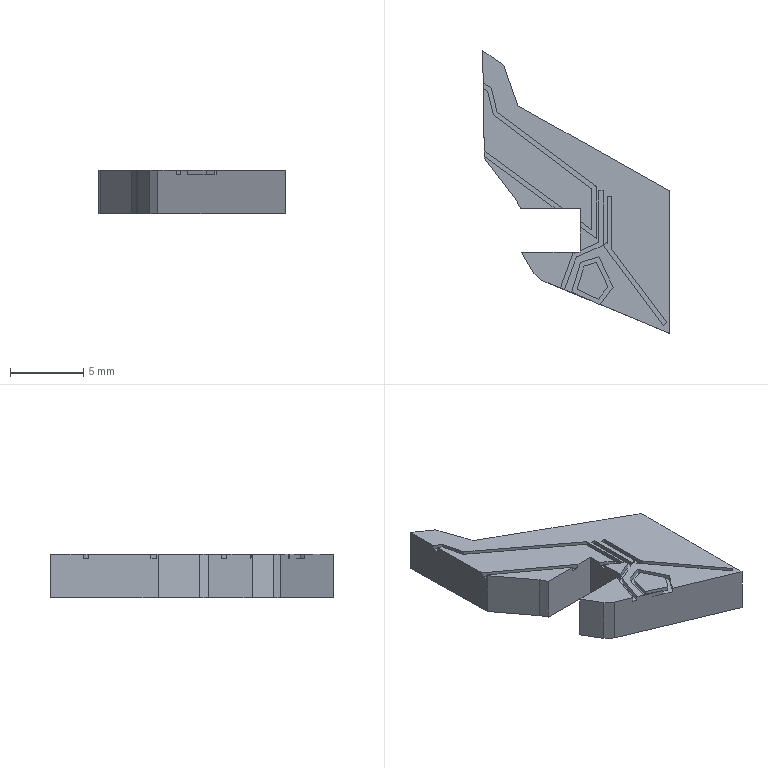Part | SolidWorks | features BaseBody 1 | 1 solid | 65 faces | box 12.769 x 19.344 x 3 mm | volume 333.771 mm3 | plane 61 | spline 4